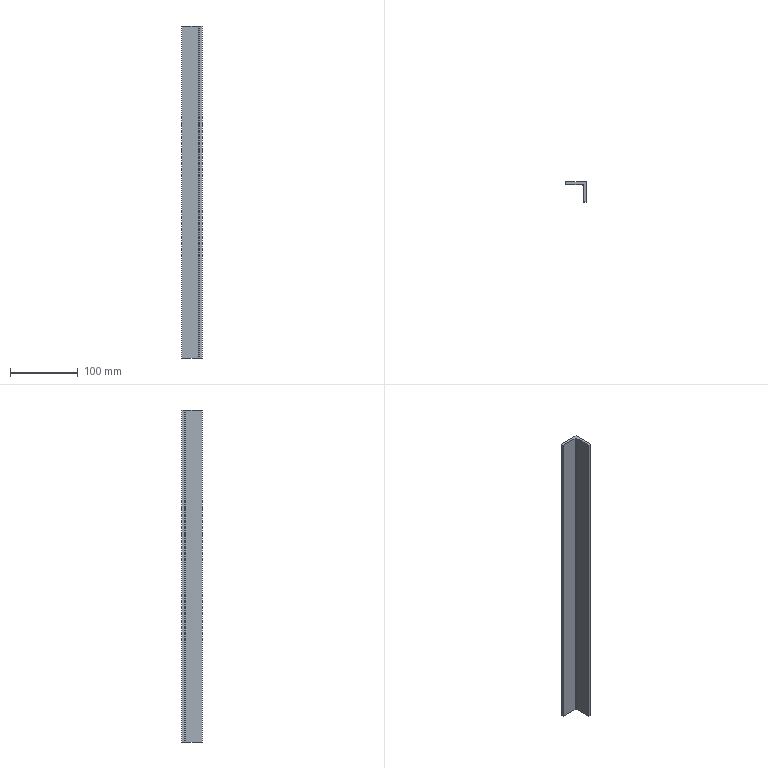Part | SolidWorks | features Extrusion 1 | 1 solid | 9 faces | box 30 x 30 x 490 mm | volume 110181 mm3 | plane 8 | cylinder 1 | commonest cylinder face diameters 4 x1
STEP:
#1=CARTESIAN_POINT('',(30.,0.,0.));
#2=VERTEX_POINT('',#1);
#3=CARTESIAN_POINT('',(30.,-30.,0.));
#4=VERTEX_POINT('',#3);
#5=CARTESIAN_POINT('',(30.,0.,0.));
#6=DIRECTION('',(0.,-1.,0.));
#7=VECTOR('',#6,1000.);
#8=LINE('',#5,#7);
#9=EDGE_CURVE('',#2,#4,#8,.T.);
#10=ORIENTED_EDGE('',*,*,#9,.F.);
#11=CARTESIAN_POINT('',(30.,0.,490.));
#12=VERTEX_POINT('',#11);
#13=CARTESIAN_POINT('',(30.,0.,490.));
#14=DIRECTION('',(0.,0.,-1.));
#15=VECTOR('',#14,1000.);
#16=LINE('',#13,#15);
#17=EDGE_CURVE('',#12,#2,#16,.T.);
#18=ORIENTED_EDGE('',*,*,#17,.F.);
#19=CARTESIAN_POINT('',(30.,-30.,490.));
#20=VERTEX_POINT('',#19);
#21=CARTESIAN_POINT('',(30.,0.,490.));
#22=DIRECTION('',(0.,-1.,0.));
#23=VECTOR('',#22,1000.);
#24=LINE('',#21,#23);
#25=EDGE_CURVE('',#12,#20,#24,.T.);
#26=ORIENTED_EDGE('',*,*,#25,.T.);
#27=CARTESIAN_POINT('',(30.,-30.,490.));
#28=DIRECTION('',(0.,0.,-1.));
#29=VECTOR('',#28,1000.);
#30=LINE('',#27,#29);
#31=EDGE_CURVE('',#20,#4,#30,.T.);
#32=ORIENTED_EDGE('',*,*,#31,.T.);
#33=EDGE_LOOP('',(#10,#18,#26,#32));
#34=FACE_OUTER_BOUND('',#33,.T.);
#35=CARTESIAN_POINT('',(30.,0.,490.));
#36=DIRECTION('',(1.,0.,0.));
#37=DIRECTION('',(0.,0.,-1.));
#38=AXIS2_PLACEMENT_3D('',#35,#36,#37);
#39=PLANE('',#38);
#40=ADVANCED_FACE('',(#34),#39,.T.);
#41=CARTESIAN_POINT('',(0.,0.,0.));
#42=VERTEX_POINT('',#41);
#43=CARTESIAN_POINT('',(0.,0.,0.));
#44=DIRECTION('',(1.,0.,0.));
#45=VECTOR('',#44,1000.);
#46=LINE('',#43,#45);
#47=EDGE_CURVE('',#42,#2,#46,.T.);
#48=ORIENTED_EDGE('',*,*,#47,.F.);
#49=CARTESIAN_POINT('',(0.,0.,490.));
#50=VERTEX_POINT('',#49);
#51=CARTESIAN_POINT('',(0.,0.,490.));
#52=DIRECTION('',(0.,0.,-1.));
#53=VECTOR('',#52,1000.);
#54=LINE('',#51,#53);
#55=EDGE_CURVE('',#50,#42,#54,.T.);
#56=ORIENTED_EDGE('',*,*,#55,.F.);
#57=CARTESIAN_POINT('',(0.,0.,490.));
#58=DIRECTION('',(1.,0.,0.));
#59=VECTOR('',#58,1000.);
#60=LINE('',#57,#59);
#61=EDGE_CURVE('',#50,#12,#60,.T.);
#62=ORIENTED_EDGE('',*,*,#61,.T.);
#63=ORIENTED_EDGE('',*,*,#17,.T.);
#64=EDGE_LOOP('',(#48,#56,#62,#63));
#65=FACE_OUTER_BOUND('',#64,.T.);
#66=CARTESIAN_POINT('',(0.,0.,490.));
#67=DIRECTION('',(0.,1.,0.));
#68=DIRECTION('',(0.,0.,1.));
#69=AXIS2_PLACEMENT_3D('',#66,#67,#68);
#70=PLANE('',#69);
#71=ADVANCED_FACE('',(#65),#70,.T.);
#72=CARTESIAN_POINT('',(0.,-4.,0.));
#73=VERTEX_POINT('',#72);
#74=CARTESIAN_POINT('',(0.,0.,0.));
#75=DIRECTION('',(0.,-1.,0.));
#76=VECTOR('',#75,1000.);
#77=LINE('',#74,#76);
#78=EDGE_CURVE('',#42,#73,#77,.T.);
#79=ORIENTED_EDGE('',*,*,#78,.T.);
#80=CARTESIAN_POINT('',(0.,-4.,490.));
#81=VERTEX_POINT('',#80);
#82=CARTESIAN_POINT('',(0.,-4.,490.));
#83=DIRECTION('',(0.,0.,-1.));
#84=VECTOR('',#83,1000.);
#85=LINE('',#82,#84);
#86=EDGE_CURVE('',#81,#73,#85,.T.);
#87=ORIENTED_EDGE('',*,*,#86,.F.);
#88=CARTESIAN_POINT('',(0.,0.,490.));
#89=DIRECTION('',(0.,-1.,0.));
#90=VECTOR('',#89,1000.);
#91=LINE('',#88,#90);
#92=EDGE_CURVE('',#50,#81,#91,.T.);
#93=ORIENTED_EDGE('',*,*,#92,.F.);
#94=ORIENTED_EDGE('',*,*,#55,.T.);
#95=EDGE_LOOP('',(#79,#87,#93,#94));
#96=FACE_OUTER_BOUND('',#95,.T.);
#97=CARTESIAN_POINT('',(0.,0.,490.));
#98=DIRECTION('',(1.,0.,0.));
#99=DIRECTION('',(0.,0.,-1.));
#100=AXIS2_PLACEMENT_3D('',#97,#98,#99);
#101=PLANE('',#100);
#102=ADVANCED_FACE('',(#96),#101,.F.);
#103=CARTESIAN_POINT('',(24.,-4.,0.));
#104=VERTEX_POINT('',#103);
#105=CARTESIAN_POINT('',(0.,-4.,0.));
#106=DIRECTION('',(1.,0.,0.));
#107=VECTOR('',#106,1000.);
#108=LINE('',#105,#107);
#109=EDGE_CURVE('',#73,#104,#108,.T.);
#110=ORIENTED_EDGE('',*,*,#109,.T.);
#111=CARTESIAN_POINT('',(24.,-4.,490.));
#112=VERTEX_POINT('',#111);
#113=CARTESIAN_POINT('',(24.,-4.,490.));
#114=DIRECTION('',(0.,0.,-1.));
#115=VECTOR('',#114,1000.);
#116=LINE('',#113,#115);
#117=EDGE_CURVE('',#112,#104,#116,.T.);
#118=ORIENTED_EDGE('',*,*,#117,.F.);
#119=CARTESIAN_POINT('',(0.,-4.,490.));
#120=DIRECTION('',(1.,0.,0.));
#121=VECTOR('',#120,1000.);
#122=LINE('',#119,#121);
#123=EDGE_CURVE('',#81,#112,#122,.T.);
#124=ORIENTED_EDGE('',*,*,#123,.F.);
#125=ORIENTED_EDGE('',*,*,#86,.T.);
#126=EDGE_LOOP('',(#110,#118,#124,#125));
#127=FACE_OUTER_BOUND('',#126,.T.);
#128=CARTESIAN_POINT('',(0.,-4.,490.));
#129=DIRECTION('',(0.,1.,0.));
#130=DIRECTION('',(-1.,0.,0.));
#131=AXIS2_PLACEMENT_3D('',#128,#129,#130);
#132=PLANE('',#131);
#133=ADVANCED_FACE('',(#127),#132,.F.);
#134=CARTESIAN_POINT('',(26.,-6.,0.));
#135=VERTEX_POINT('',#134);
#136=CARTESIAN_POINT('',(24.,-6.,0.));
#137=DIRECTION('',(0.,0.,-1.));
#138=DIRECTION('',(-1.,0.,0.));
#139=AXIS2_PLACEMENT_3D('',#136,#137,#138);
#140=CIRCLE('',#139,2.);
#141=EDGE_CURVE('',#104,#135,#140,.T.);
#142=ORIENTED_EDGE('',*,*,#141,.T.);
#143=CARTESIAN_POINT('',(26.,-6.,490.));
#144=VERTEX_POINT('',#143);
#145=CARTESIAN_POINT('',(26.,-6.,490.));
#146=DIRECTION('',(0.,0.,-1.));
#147=VECTOR('',#146,1000.);
#148=LINE('',#145,#147);
#149=EDGE_CURVE('',#144,#135,#148,.T.);
#150=ORIENTED_EDGE('',*,*,#149,.F.);
#151=CARTESIAN_POINT('',(24.,-6.,490.));
#152=DIRECTION('',(0.,0.,-1.));
#153=DIRECTION('',(-1.,0.,0.));
#154=AXIS2_PLACEMENT_3D('',#151,#152,#153);
#155=CIRCLE('',#154,2.);
#156=EDGE_CURVE('',#112,#144,#155,.T.);
#157=ORIENTED_EDGE('',*,*,#156,.F.);
#158=ORIENTED_EDGE('',*,*,#117,.T.);
#159=EDGE_LOOP('',(#142,#150,#157,#158));
#160=FACE_OUTER_BOUND('',#159,.T.);
#161=CARTESIAN_POINT('',(24.,-6.,490.));
#162=DIRECTION('',(0.,0.,-1.));
#163=DIRECTION('',(-1.,0.,0.));
#164=AXIS2_PLACEMENT_3D('',#161,#162,#163);
#165=CYLINDRICAL_SURFACE('',#164,2.);
#166=ADVANCED_FACE('',(#160),#165,.F.);
#167=CARTESIAN_POINT('',(26.,-30.,0.));
#168=VERTEX_POINT('',#167);
#169=CARTESIAN_POINT('',(26.,-6.,0.));
#170=DIRECTION('',(0.,-1.,0.));
#171=VECTOR('',#170,1000.);
#172=LINE('',#169,#171);
#173=EDGE_CURVE('',#135,#168,#172,.T.);
#174=ORIENTED_EDGE('',*,*,#173,.T.);
#175=CARTESIAN_POINT('',(26.,-30.,490.));
#176=VERTEX_POINT('',#175);
#177=CARTESIAN_POINT('',(26.,-30.,490.));
#178=DIRECTION('',(0.,0.,-1.));
#179=VECTOR('',#178,1000.);
#180=LINE('',#177,#179);
#181=EDGE_CURVE('',#176,#168,#180,.T.);
#182=ORIENTED_EDGE('',*,*,#181,.F.);
#183=CARTESIAN_POINT('',(26.,-6.,490.));
#184=DIRECTION('',(0.,-1.,0.));
#185=VECTOR('',#184,1000.);
#186=LINE('',#183,#185);
#187=EDGE_CURVE('',#144,#176,#186,.T.);
#188=ORIENTED_EDGE('',*,*,#187,.F.);
#189=ORIENTED_EDGE('',*,*,#149,.T.);
#190=EDGE_LOOP('',(#174,#182,#188,#189));
#191=FACE_OUTER_BOUND('',#190,.T.);
#192=CARTESIAN_POINT('',(26.,-6.,490.));
#193=DIRECTION('',(1.,0.,0.));
#194=DIRECTION('',(0.,0.,-1.));
#195=AXIS2_PLACEMENT_3D('',#192,#193,#194);
#196=PLANE('',#195);
#197=ADVANCED_FACE('',(#191),#196,.F.);
#198=CARTESIAN_POINT('',(30.,-30.,0.));
#199=DIRECTION('',(-1.,0.,0.));
#200=VECTOR('',#199,1000.);
#201=LINE('',#198,#200);
#202=EDGE_CURVE('',#4,#168,#201,.T.);
#203=ORIENTED_EDGE('',*,*,#202,.F.);
#204=ORIENTED_EDGE('',*,*,#31,.F.);
#205=CARTESIAN_POINT('',(30.,-30.,490.));
#206=DIRECTION('',(-1.,0.,0.));
#207=VECTOR('',#206,1000.);
#208=LINE('',#205,#207);
#209=EDGE_CURVE('',#20,#176,#208,.T.);
#210=ORIENTED_EDGE('',*,*,#209,.T.);
#211=ORIENTED_EDGE('',*,*,#181,.T.);
#212=EDGE_LOOP('',(#203,#204,#210,#211));
#213=FACE_OUTER_BOUND('',#212,.T.);
#214=CARTESIAN_POINT('',(30.,-30.,490.));
#215=DIRECTION('',(0.,-1.,0.));
#216=DIRECTION('',(0.,0.,-1.));
#217=AXIS2_PLACEMENT_3D('',#214,#215,#216);
#218=PLANE('',#217);
#219=ADVANCED_FACE('',(#213),#218,.T.);
#220=ORIENTED_EDGE('',*,*,#25,.F.);
#221=ORIENTED_EDGE('',*,*,#61,.F.);
#222=ORIENTED_EDGE('',*,*,#92,.T.);
#223=ORIENTED_EDGE('',*,*,#123,.T.);
#224=ORIENTED_EDGE('',*,*,#156,.T.);
#225=ORIENTED_EDGE('',*,*,#187,.T.);
#226=ORIENTED_EDGE('',*,*,#209,.F.);
#227=EDGE_LOOP('',(#220,#221,#222,#223,#224,#225,#226));
#228=FACE_OUTER_BOUND('',#227,.T.);
#229=CARTESIAN_POINT('',(24.,-6.,490.));
#230=DIRECTION('',(0.,0.,-1.));
#231=DIRECTION('',(-1.,0.,0.));
#232=AXIS2_PLACEMENT_3D('',#229,#230,#231);
#233=PLANE('',#232);
#234=ADVANCED_FACE('',(#228),#233,.F.);
#235=ORIENTED_EDGE('',*,*,#9,.T.);
#236=ORIENTED_EDGE('',*,*,#202,.T.);
#237=ORIENTED_EDGE('',*,*,#173,.F.);
#238=ORIENTED_EDGE('',*,*,#141,.F.);
#239=ORIENTED_EDGE('',*,*,#109,.F.);
#240=ORIENTED_EDGE('',*,*,#78,.F.);
#241=ORIENTED_EDGE('',*,*,#47,.T.);
#242=EDGE_LOOP('',(#235,#236,#237,#238,#239,#240,#241));
#243=FACE_OUTER_BOUND('',#242,.T.);
#244=CARTESIAN_POINT('',(24.,-6.,0.));
#245=DIRECTION('',(0.,0.,-1.));
#246=DIRECTION('',(-1.,0.,0.));
#247=AXIS2_PLACEMENT_3D('',#244,#245,#246);
#248=PLANE('',#247);
#249=ADVANCED_FACE('',(#243),#248,.T.);
#250=CLOSED_SHELL('',(#40,#71,#102,#133,#166,#197,#219,#234,#249));
#251=MANIFOLD_SOLID_BREP('',#250);
#252=CARTESIAN_POINT('',(0.,0.,0.));
#253=DIRECTION('',(0.,0.,1.));
#254=DIRECTION('',(1.,0.,0.));
#255=AXIS2_PLACEMENT_3D('',#252,#253,#254);
#256=(LENGTH_UNIT()NAMED_UNIT(*)SI_UNIT(.MILLI.,.METRE.));
#257=UNCERTAINTY_MEASURE_WITH_UNIT(LENGTH_MEASURE(0.00001),#256,'','');
#258=(NAMED_UNIT(*)PLANE_ANGLE_UNIT()SI_UNIT($,.RADIAN.));
#259=(NAMED_UNIT(*)SI_UNIT($,.STERADIAN.)SOLID_ANGLE_UNIT());
#260=(GEOMETRIC_REPRESENTATION_CONTEXT(3)GLOBAL_UNCERTAINTY_ASSIGNED_CONTEXT((#257))GLOBAL_UNIT_ASSIGNED_CONTEXT((#256,#258,#259))REPRESENTATION_CONTEXT('',''));
#261=ADVANCED_BREP_SHAPE_REPRESENTATION('',(#251,#255),#260);